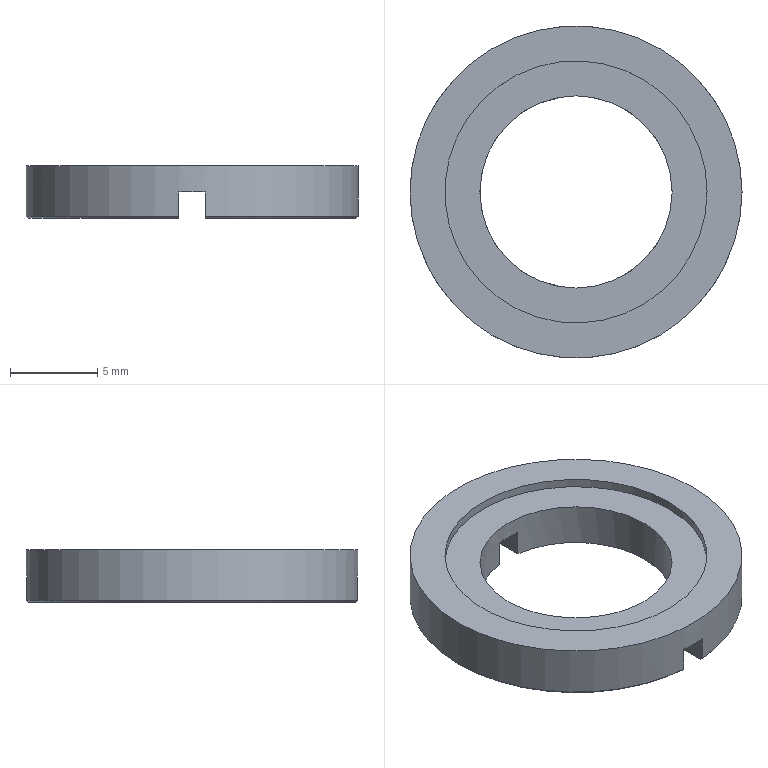Part | NX | 1 solid | 15 faces | box 19 x 19 x 3 mm | volume 506.207 mm3 | plane 10 | cylinder 3 | cone 2 | commonest cylinder face diameters 11 x1 15 x1 19 x1
STEP:
#1=CARTESIAN_POINT('',(-0.75,9.47,1.5));
#2=VERTEX_POINT('',#1);
#3=CARTESIAN_POINT('',(0.75,9.47,1.5));
#4=VERTEX_POINT('',#3);
#5=CARTESIAN_POINT('',(0.,0.,1.5));
#6=DIRECTION('',(0.,0.,-1.));
#7=DIRECTION('',(-1.,0.,0.));
#8=AXIS2_PLACEMENT_3D('',#5,#6,#7);
#9=CIRCLE('',#8,9.5);
#10=EDGE_CURVE('',#2,#4,#9,.T.);
#11=ORIENTED_EDGE('',*,*,#10,.F.);
#12=CARTESIAN_POINT('',(-0.75,9.47,0.12));
#13=VERTEX_POINT('',#12);
#14=CARTESIAN_POINT('',(-0.75,9.47,1.5));
#15=DIRECTION('',(0.,0.,1.));
#16=VECTOR('',#15,1000.);
#17=LINE('',#14,#16);
#18=EDGE_CURVE('',#2,#13,#17,.F.);
#19=ORIENTED_EDGE('',*,*,#18,.T.);
#20=CARTESIAN_POINT('',(-0.75,-9.47,0.12));
#21=VERTEX_POINT('',#20);
#22=CARTESIAN_POINT('',(0.,0.,0.12));
#23=DIRECTION('',(0.,0.,-1.));
#24=DIRECTION('',(-1.,0.,0.));
#25=AXIS2_PLACEMENT_3D('',#22,#23,#24);
#26=CIRCLE('',#25,9.5);
#27=EDGE_CURVE('',#13,#21,#26,.F.);
#28=ORIENTED_EDGE('',*,*,#27,.T.);
#29=CARTESIAN_POINT('',(-0.75,-9.47,1.5));
#30=VERTEX_POINT('',#29);
#31=CARTESIAN_POINT('',(-0.75,-9.47,1.5));
#32=DIRECTION('',(0.,0.,1.));
#33=VECTOR('',#32,1000.);
#34=LINE('',#31,#33);
#35=EDGE_CURVE('',#21,#30,#34,.T.);
#36=ORIENTED_EDGE('',*,*,#35,.T.);
#37=CARTESIAN_POINT('',(0.75,-9.47,1.5));
#38=VERTEX_POINT('',#37);
#39=CARTESIAN_POINT('',(0.,0.,1.5));
#40=DIRECTION('',(0.,0.,-1.));
#41=DIRECTION('',(-1.,0.,0.));
#42=AXIS2_PLACEMENT_3D('',#39,#40,#41);
#43=CIRCLE('',#42,9.5);
#44=EDGE_CURVE('',#38,#30,#43,.T.);
#45=ORIENTED_EDGE('',*,*,#44,.F.);
#46=CARTESIAN_POINT('',(0.75,-9.47,0.12));
#47=VERTEX_POINT('',#46);
#48=CARTESIAN_POINT('',(0.75,-9.47,1.5));
#49=DIRECTION('',(0.,0.,-1.));
#50=VECTOR('',#49,1000.);
#51=LINE('',#48,#50);
#52=EDGE_CURVE('',#38,#47,#51,.T.);
#53=ORIENTED_EDGE('',*,*,#52,.T.);
#54=CARTESIAN_POINT('',(0.75,9.47,0.12));
#55=VERTEX_POINT('',#54);
#56=CARTESIAN_POINT('',(0.,0.,0.12));
#57=DIRECTION('',(0.,0.,-1.));
#58=DIRECTION('',(-1.,0.,0.));
#59=AXIS2_PLACEMENT_3D('',#56,#57,#58);
#60=CIRCLE('',#59,9.5);
#61=EDGE_CURVE('',#47,#55,#60,.F.);
#62=ORIENTED_EDGE('',*,*,#61,.T.);
#63=CARTESIAN_POINT('',(0.75,9.47,1.5));
#64=DIRECTION('',(0.,0.,-1.));
#65=VECTOR('',#64,1000.);
#66=LINE('',#63,#65);
#67=EDGE_CURVE('',#55,#4,#66,.F.);
#68=ORIENTED_EDGE('',*,*,#67,.T.);
#69=EDGE_LOOP('',(#11,#19,#28,#36,#45,#53,#62,#68));
#70=FACE_BOUND('',#69,.T.);
#71=CARTESIAN_POINT('',(-9.5,0.,3.));
#72=VERTEX_POINT('',#71);
#73=CARTESIAN_POINT('',(0.,0.,3.));
#74=DIRECTION('',(0.,0.,-1.));
#75=DIRECTION('',(-1.,0.,0.));
#76=AXIS2_PLACEMENT_3D('',#73,#74,#75);
#77=CIRCLE('',#76,9.5);
#78=EDGE_CURVE('',#72,#72,#77,.T.);
#79=ORIENTED_EDGE('',*,*,#78,.T.);
#80=EDGE_LOOP('',(#79));
#81=FACE_BOUND('',#80,.T.);
#82=CARTESIAN_POINT('',(0.,0.,3.));
#83=DIRECTION('',(0.,0.,-1.));
#84=DIRECTION('',(-1.,0.,0.));
#85=AXIS2_PLACEMENT_3D('',#82,#83,#84);
#86=CYLINDRICAL_SURFACE('',#85,9.5);
#87=ADVANCED_FACE('',(#70,#81),#86,.T.);
#88=ORIENTED_EDGE('',*,*,#61,.F.);
#89=CARTESIAN_POINT('',(0.75,-9.35,0.));
#90=VERTEX_POINT('',#89);
#91=CARTESIAN_POINT('',(0.75,-9.47,0.12));
#92=CARTESIAN_POINT('',(0.75,-9.43,0.08));
#93=CARTESIAN_POINT('',(0.75,-9.39,0.04));
#94=CARTESIAN_POINT('',(0.75,-9.35,0.));
#95=B_SPLINE_CURVE_WITH_KNOTS('',3,(#91,#92,#93,#94),.UNSPECIFIED.,.F.,.F.,(4,4),(0.,0.00017),.UNSPECIFIED.);
#96=EDGE_CURVE('',#47,#90,#95,.T.);
#97=ORIENTED_EDGE('',*,*,#96,.T.);
#98=CARTESIAN_POINT('',(0.75,9.35,0.));
#99=VERTEX_POINT('',#98);
#100=CARTESIAN_POINT('',(0.,0.,0.));
#101=DIRECTION('',(0.,0.,1.));
#102=DIRECTION('',(0.,-1.,0.));
#103=AXIS2_PLACEMENT_3D('',#100,#101,#102);
#104=CIRCLE('',#103,9.38);
#105=EDGE_CURVE('',#90,#99,#104,.T.);
#106=ORIENTED_EDGE('',*,*,#105,.T.);
#107=CARTESIAN_POINT('',(0.75,9.35,0.));
#108=CARTESIAN_POINT('',(0.75,9.39,0.04));
#109=CARTESIAN_POINT('',(0.75,9.43,0.08));
#110=CARTESIAN_POINT('',(0.75,9.47,0.12));
#111=B_SPLINE_CURVE_WITH_KNOTS('',3,(#107,#108,#109,#110),.UNSPECIFIED.,.F.,.F.,(4,4),(0.,0.00017),.UNSPECIFIED.);
#112=EDGE_CURVE('',#99,#55,#111,.T.);
#113=ORIENTED_EDGE('',*,*,#112,.T.);
#114=EDGE_LOOP('',(#88,#97,#106,#113));
#115=FACE_BOUND('',#114,.T.);
#116=CARTESIAN_POINT('',(0.,0.,0.12));
#117=DIRECTION('',(0.,0.,1.));
#118=DIRECTION('',(0.,-1.,0.));
#119=AXIS2_PLACEMENT_3D('',#116,#117,#118);
#120=CONICAL_SURFACE('',#119,9.5,0.7854);
#121=ADVANCED_FACE('',(#115),#120,.T.);
#122=CARTESIAN_POINT('',(-0.75,9.35,0.));
#123=VERTEX_POINT('',#122);
#124=CARTESIAN_POINT('',(-0.75,9.47,0.12));
#125=CARTESIAN_POINT('',(-0.75,9.43,0.08));
#126=CARTESIAN_POINT('',(-0.75,9.39,0.04));
#127=CARTESIAN_POINT('',(-0.75,9.35,0.));
#128=B_SPLINE_CURVE_WITH_KNOTS('',3,(#124,#125,#126,#127),.UNSPECIFIED.,.F.,.F.,(4,4),(0.,0.00017),.UNSPECIFIED.);
#129=EDGE_CURVE('',#13,#123,#128,.T.);
#130=ORIENTED_EDGE('',*,*,#129,.T.);
#131=CARTESIAN_POINT('',(-0.75,-9.35,0.));
#132=VERTEX_POINT('',#131);
#133=CARTESIAN_POINT('',(0.,0.,0.));
#134=DIRECTION('',(0.,0.,1.));
#135=DIRECTION('',(0.,-1.,0.));
#136=AXIS2_PLACEMENT_3D('',#133,#134,#135);
#137=CIRCLE('',#136,9.38);
#138=EDGE_CURVE('',#123,#132,#137,.T.);
#139=ORIENTED_EDGE('',*,*,#138,.T.);
#140=CARTESIAN_POINT('',(-0.75,-9.35,0.));
#141=CARTESIAN_POINT('',(-0.75,-9.39,0.04));
#142=CARTESIAN_POINT('',(-0.75,-9.43,0.08));
#143=CARTESIAN_POINT('',(-0.75,-9.47,0.12));
#144=B_SPLINE_CURVE_WITH_KNOTS('',3,(#140,#141,#142,#143),.UNSPECIFIED.,.F.,.F.,(4,4),(0.,0.00017),.UNSPECIFIED.);
#145=EDGE_CURVE('',#132,#21,#144,.T.);
#146=ORIENTED_EDGE('',*,*,#145,.T.);
#147=ORIENTED_EDGE('',*,*,#27,.F.);
#148=EDGE_LOOP('',(#130,#139,#146,#147));
#149=FACE_BOUND('',#148,.T.);
#150=CARTESIAN_POINT('',(0.,0.,0.12));
#151=DIRECTION('',(0.,0.,1.));
#152=DIRECTION('',(0.,-1.,0.));
#153=AXIS2_PLACEMENT_3D('',#150,#151,#152);
#154=CONICAL_SURFACE('',#153,9.5,0.7854);
#155=ADVANCED_FACE('',(#149),#154,.T.);
#156=CARTESIAN_POINT('',(7.5,0.,3.));
#157=VERTEX_POINT('',#156);
#158=CARTESIAN_POINT('',(0.,0.,3.));
#159=DIRECTION('',(0.,0.,1.));
#160=DIRECTION('',(1.,0.,0.));
#161=AXIS2_PLACEMENT_3D('',#158,#159,#160);
#162=CIRCLE('',#161,7.5);
#163=EDGE_CURVE('',#157,#157,#162,.F.);
#164=ORIENTED_EDGE('',*,*,#163,.T.);
#165=EDGE_LOOP('',(#164));
#166=FACE_BOUND('',#165,.T.);
#167=ORIENTED_EDGE('',*,*,#78,.F.);
#168=EDGE_LOOP('',(#167));
#169=FACE_BOUND('',#168,.T.);
#170=CARTESIAN_POINT('',(0.,0.,3.));
#171=DIRECTION('',(0.,0.,1.));
#172=DIRECTION('',(1.,0.,0.));
#173=AXIS2_PLACEMENT_3D('',#170,#171,#172);
#174=PLANE('',#173);
#175=ADVANCED_FACE('',(#166,#169),#174,.T.);
#176=CARTESIAN_POINT('',(0.75,-5.449,0.));
#177=VERTEX_POINT('',#176);
#178=CARTESIAN_POINT('',(0.75,0.,0.));
#179=DIRECTION('',(0.,1.,0.));
#180=VECTOR('',#179,1000.);
#181=LINE('',#178,#180);
#182=EDGE_CURVE('',#177,#90,#181,.F.);
#183=ORIENTED_EDGE('',*,*,#182,.F.);
#184=CARTESIAN_POINT('',(0.75,5.449,0.));
#185=VERTEX_POINT('',#184);
#186=CARTESIAN_POINT('',(0.,0.,0.));
#187=DIRECTION('',(0.,0.,1.));
#188=DIRECTION('',(1.,0.,0.));
#189=AXIS2_PLACEMENT_3D('',#186,#187,#188);
#190=CIRCLE('',#189,5.5);
#191=EDGE_CURVE('',#185,#177,#190,.F.);
#192=ORIENTED_EDGE('',*,*,#191,.F.);
#193=CARTESIAN_POINT('',(0.75,0.,0.));
#194=DIRECTION('',(0.,1.,0.));
#195=VECTOR('',#194,1000.);
#196=LINE('',#193,#195);
#197=EDGE_CURVE('',#99,#185,#196,.F.);
#198=ORIENTED_EDGE('',*,*,#197,.F.);
#199=ORIENTED_EDGE('',*,*,#105,.F.);
#200=EDGE_LOOP('',(#183,#192,#198,#199));
#201=FACE_BOUND('',#200,.T.);
#202=CARTESIAN_POINT('',(0.,0.,0.));
#203=DIRECTION('',(0.,0.,1.));
#204=DIRECTION('',(1.,0.,0.));
#205=AXIS2_PLACEMENT_3D('',#202,#203,#204);
#206=PLANE('',#205);
#207=ADVANCED_FACE('',(#201),#206,.F.);
#208=CARTESIAN_POINT('',(-0.75,5.449,0.));
#209=VERTEX_POINT('',#208);
#210=CARTESIAN_POINT('',(-0.75,0.,0.));
#211=DIRECTION('',(0.,1.,0.));
#212=VECTOR('',#211,1000.);
#213=LINE('',#210,#212);
#214=EDGE_CURVE('',#209,#123,#213,.T.);
#215=ORIENTED_EDGE('',*,*,#214,.F.);
#216=CARTESIAN_POINT('',(-0.75,-5.449,0.));
#217=VERTEX_POINT('',#216);
#218=CARTESIAN_POINT('',(0.,0.,0.));
#219=DIRECTION('',(0.,0.,1.));
#220=DIRECTION('',(1.,0.,0.));
#221=AXIS2_PLACEMENT_3D('',#218,#219,#220);
#222=CIRCLE('',#221,5.5);
#223=EDGE_CURVE('',#217,#209,#222,.F.);
#224=ORIENTED_EDGE('',*,*,#223,.F.);
#225=CARTESIAN_POINT('',(-0.75,0.,0.));
#226=DIRECTION('',(0.,1.,0.));
#227=VECTOR('',#226,1000.);
#228=LINE('',#225,#227);
#229=EDGE_CURVE('',#132,#217,#228,.T.);
#230=ORIENTED_EDGE('',*,*,#229,.F.);
#231=ORIENTED_EDGE('',*,*,#138,.F.);
#232=EDGE_LOOP('',(#215,#224,#230,#231));
#233=FACE_BOUND('',#232,.T.);
#234=CARTESIAN_POINT('',(0.,0.,0.));
#235=DIRECTION('',(0.,0.,1.));
#236=DIRECTION('',(1.,0.,0.));
#237=AXIS2_PLACEMENT_3D('',#234,#235,#236);
#238=PLANE('',#237);
#239=ADVANCED_FACE('',(#233),#238,.F.);
#240=ORIENTED_EDGE('',*,*,#163,.F.);
#241=EDGE_LOOP('',(#240));
#242=FACE_BOUND('',#241,.T.);
#243=CARTESIAN_POINT('',(7.5,0.,2.5));
#244=VERTEX_POINT('',#243);
#245=CARTESIAN_POINT('',(0.,0.,2.5));
#246=DIRECTION('',(0.,0.,1.));
#247=DIRECTION('',(1.,0.,0.));
#248=AXIS2_PLACEMENT_3D('',#245,#246,#247);
#249=CIRCLE('',#248,7.5);
#250=EDGE_CURVE('',#244,#244,#249,.T.);
#251=ORIENTED_EDGE('',*,*,#250,.F.);
#252=EDGE_LOOP('',(#251));
#253=FACE_BOUND('',#252,.T.);
#254=CARTESIAN_POINT('',(0.,0.,2.5));
#255=DIRECTION('',(0.,0.,1.));
#256=DIRECTION('',(1.,0.,0.));
#257=AXIS2_PLACEMENT_3D('',#254,#255,#256);
#258=CYLINDRICAL_SURFACE('',#257,7.5);
#259=ADVANCED_FACE('',(#242,#253),#258,.F.);
#260=ORIENTED_EDGE('',*,*,#96,.F.);
#261=ORIENTED_EDGE('',*,*,#52,.F.);
#262=CARTESIAN_POINT('',(0.75,-5.449,1.5));
#263=VERTEX_POINT('',#262);
#264=CARTESIAN_POINT('',(0.75,10.835,1.5));
#265=DIRECTION('',(0.,1.,0.));
#266=VECTOR('',#265,1000.);
#267=LINE('',#264,#266);
#268=EDGE_CURVE('',#263,#38,#267,.F.);
#269=ORIENTED_EDGE('',*,*,#268,.F.);
#270=CARTESIAN_POINT('',(0.75,-5.449,1.5));
#271=DIRECTION('',(0.,0.,-1.));
#272=VECTOR('',#271,1000.);
#273=LINE('',#270,#272);
#274=EDGE_CURVE('',#177,#263,#273,.F.);
#275=ORIENTED_EDGE('',*,*,#274,.F.);
#276=ORIENTED_EDGE('',*,*,#182,.T.);
#277=EDGE_LOOP('',(#260,#261,#269,#275,#276));
#278=FACE_BOUND('',#277,.T.);
#279=CARTESIAN_POINT('',(0.75,10.835,1.5));
#280=DIRECTION('',(1.,0.,0.));
#281=DIRECTION('',(0.,0.,-1.));
#282=AXIS2_PLACEMENT_3D('',#279,#280,#281);
#283=PLANE('',#282);
#284=ADVANCED_FACE('',(#278),#283,.F.);
#285=CARTESIAN_POINT('',(5.5,0.,2.5));
#286=VERTEX_POINT('',#285);
#287=CARTESIAN_POINT('',(0.,0.,2.5));
#288=DIRECTION('',(0.,0.,1.));
#289=DIRECTION('',(1.,0.,0.));
#290=AXIS2_PLACEMENT_3D('',#287,#288,#289);
#291=CIRCLE('',#290,5.5);
#292=EDGE_CURVE('',#286,#286,#291,.F.);
#293=ORIENTED_EDGE('',*,*,#292,.F.);
#294=EDGE_LOOP('',(#293));
#295=FACE_BOUND('',#294,.T.);
#296=ORIENTED_EDGE('',*,*,#274,.T.);
#297=CARTESIAN_POINT('',(-0.75,-5.449,1.5));
#298=VERTEX_POINT('',#297);
#299=CARTESIAN_POINT('',(0.,0.,1.5));
#300=DIRECTION('',(0.,0.,1.));
#301=DIRECTION('',(1.,0.,0.));
#302=AXIS2_PLACEMENT_3D('',#299,#300,#301);
#303=CIRCLE('',#302,5.5);
#304=EDGE_CURVE('',#298,#263,#303,.T.);
#305=ORIENTED_EDGE('',*,*,#304,.F.);
#306=CARTESIAN_POINT('',(-0.75,-5.449,0.));
#307=DIRECTION('',(0.,0.,1.));
#308=VECTOR('',#307,1000.);
#309=LINE('',#306,#308);
#310=EDGE_CURVE('',#217,#298,#309,.T.);
#311=ORIENTED_EDGE('',*,*,#310,.F.);
#312=ORIENTED_EDGE('',*,*,#223,.T.);
#313=CARTESIAN_POINT('',(-0.75,5.449,1.5));
#314=VERTEX_POINT('',#313);
#315=CARTESIAN_POINT('',(-0.75,5.449,0.));
#316=DIRECTION('',(0.,0.,1.));
#317=VECTOR('',#316,1000.);
#318=LINE('',#315,#317);
#319=EDGE_CURVE('',#314,#209,#318,.F.);
#320=ORIENTED_EDGE('',*,*,#319,.F.);
#321=CARTESIAN_POINT('',(0.75,5.449,1.5));
#322=VERTEX_POINT('',#321);
#323=CARTESIAN_POINT('',(0.,0.,1.5));
#324=DIRECTION('',(0.,0.,1.));
#325=DIRECTION('',(1.,0.,0.));
#326=AXIS2_PLACEMENT_3D('',#323,#324,#325);
#327=CIRCLE('',#326,5.5);
#328=EDGE_CURVE('',#322,#314,#327,.T.);
#329=ORIENTED_EDGE('',*,*,#328,.F.);
#330=CARTESIAN_POINT('',(0.75,5.449,0.));
#331=DIRECTION('',(0.,0.,1.));
#332=VECTOR('',#331,1000.);
#333=LINE('',#330,#332);
#334=EDGE_CURVE('',#185,#322,#333,.T.);
#335=ORIENTED_EDGE('',*,*,#334,.F.);
#336=ORIENTED_EDGE('',*,*,#191,.T.);
#337=EDGE_LOOP('',(#296,#305,#311,#312,#320,#329,#335,#336));
#338=FACE_BOUND('',#337,.T.);
#339=CARTESIAN_POINT('',(0.,0.,0.));
#340=DIRECTION('',(0.,0.,1.));
#341=DIRECTION('',(1.,0.,0.));
#342=AXIS2_PLACEMENT_3D('',#339,#340,#341);
#343=CYLINDRICAL_SURFACE('',#342,5.5);
#344=ADVANCED_FACE('',(#295,#338),#343,.F.);
#345=ORIENTED_EDGE('',*,*,#67,.F.);
#346=ORIENTED_EDGE('',*,*,#112,.F.);
#347=ORIENTED_EDGE('',*,*,#197,.T.);
#348=ORIENTED_EDGE('',*,*,#334,.T.);
#349=CARTESIAN_POINT('',(0.75,10.835,1.5));
#350=DIRECTION('',(0.,1.,0.));
#351=VECTOR('',#350,1000.);
#352=LINE('',#349,#351);
#353=EDGE_CURVE('',#4,#322,#352,.F.);
#354=ORIENTED_EDGE('',*,*,#353,.F.);
#355=EDGE_LOOP('',(#345,#346,#347,#348,#354));
#356=FACE_BOUND('',#355,.T.);
#357=CARTESIAN_POINT('',(0.75,10.835,1.5));
#358=DIRECTION('',(1.,0.,0.));
#359=DIRECTION('',(0.,0.,-1.));
#360=AXIS2_PLACEMENT_3D('',#357,#358,#359);
#361=PLANE('',#360);
#362=ADVANCED_FACE('',(#356),#361,.F.);
#363=ORIENTED_EDGE('',*,*,#129,.F.);
#364=ORIENTED_EDGE('',*,*,#18,.F.);
#365=CARTESIAN_POINT('',(-0.75,10.835,1.5));
#366=DIRECTION('',(0.,1.,0.));
#367=VECTOR('',#366,1000.);
#368=LINE('',#365,#367);
#369=EDGE_CURVE('',#314,#2,#368,.T.);
#370=ORIENTED_EDGE('',*,*,#369,.F.);
#371=ORIENTED_EDGE('',*,*,#319,.T.);
#372=ORIENTED_EDGE('',*,*,#214,.T.);
#373=EDGE_LOOP('',(#363,#364,#370,#371,#372));
#374=FACE_BOUND('',#373,.T.);
#375=CARTESIAN_POINT('',(-0.75,10.835,1.5));
#376=DIRECTION('',(-1.,0.,0.));
#377=DIRECTION('',(0.,0.,1.));
#378=AXIS2_PLACEMENT_3D('',#375,#376,#377);
#379=PLANE('',#378);
#380=ADVANCED_FACE('',(#374),#379,.F.);
#381=ORIENTED_EDGE('',*,*,#35,.F.);
#382=ORIENTED_EDGE('',*,*,#145,.F.);
#383=ORIENTED_EDGE('',*,*,#229,.T.);
#384=ORIENTED_EDGE('',*,*,#310,.T.);
#385=CARTESIAN_POINT('',(-0.75,10.835,1.5));
#386=DIRECTION('',(0.,1.,0.));
#387=VECTOR('',#386,1000.);
#388=LINE('',#385,#387);
#389=EDGE_CURVE('',#30,#298,#388,.T.);
#390=ORIENTED_EDGE('',*,*,#389,.F.);
#391=EDGE_LOOP('',(#381,#382,#383,#384,#390));
#392=FACE_BOUND('',#391,.T.);
#393=CARTESIAN_POINT('',(-0.75,10.835,1.5));
#394=DIRECTION('',(-1.,0.,0.));
#395=DIRECTION('',(0.,0.,1.));
#396=AXIS2_PLACEMENT_3D('',#393,#394,#395);
#397=PLANE('',#396);
#398=ADVANCED_FACE('',(#392),#397,.F.);
#399=ORIENTED_EDGE('',*,*,#292,.T.);
#400=EDGE_LOOP('',(#399));
#401=FACE_BOUND('',#400,.T.);
#402=ORIENTED_EDGE('',*,*,#250,.T.);
#403=EDGE_LOOP('',(#402));
#404=FACE_BOUND('',#403,.T.);
#405=CARTESIAN_POINT('',(0.,0.,2.5));
#406=DIRECTION('',(0.,0.,1.));
#407=DIRECTION('',(1.,0.,0.));
#408=AXIS2_PLACEMENT_3D('',#405,#406,#407);
#409=PLANE('',#408);
#410=ADVANCED_FACE('',(#401,#404),#409,.T.);
#411=ORIENTED_EDGE('',*,*,#304,.T.);
#412=ORIENTED_EDGE('',*,*,#268,.T.);
#413=ORIENTED_EDGE('',*,*,#44,.T.);
#414=ORIENTED_EDGE('',*,*,#389,.T.);
#415=EDGE_LOOP('',(#411,#412,#413,#414));
#416=FACE_BOUND('',#415,.T.);
#417=CARTESIAN_POINT('',(0.75,-11.779,1.5));
#418=DIRECTION('',(0.,0.,-1.));
#419=DIRECTION('',(-1.,0.,0.));
#420=AXIS2_PLACEMENT_3D('',#417,#418,#419);
#421=PLANE('',#420);
#422=ADVANCED_FACE('',(#416),#421,.T.);
#423=ORIENTED_EDGE('',*,*,#328,.T.);
#424=ORIENTED_EDGE('',*,*,#369,.T.);
#425=ORIENTED_EDGE('',*,*,#10,.T.);
#426=ORIENTED_EDGE('',*,*,#353,.T.);
#427=EDGE_LOOP('',(#423,#424,#425,#426));
#428=FACE_BOUND('',#427,.T.);
#429=CARTESIAN_POINT('',(0.75,-11.779,1.5));
#430=DIRECTION('',(0.,0.,-1.));
#431=DIRECTION('',(-1.,0.,0.));
#432=AXIS2_PLACEMENT_3D('',#429,#430,#431);
#433=PLANE('',#432);
#434=ADVANCED_FACE('',(#428),#433,.T.);
#435=CLOSED_SHELL('',(#87,#121,#155,#175,#207,#239,#259,#284,#344,#362,#380,#398,#410,#422,#434));
#436=MANIFOLD_SOLID_BREP('',#435);
#437=(LENGTH_UNIT()NAMED_UNIT(*)SI_UNIT(.MILLI.,.METRE.));
#438=UNCERTAINTY_MEASURE_WITH_UNIT(LENGTH_MEASURE(0.0508),#437,'','');
#439=(NAMED_UNIT(*)PLANE_ANGLE_UNIT()SI_UNIT($,.RADIAN.));
#440=(NAMED_UNIT(*)SI_UNIT($,.STERADIAN.)SOLID_ANGLE_UNIT());
#441=(GEOMETRIC_REPRESENTATION_CONTEXT(3)GLOBAL_UNCERTAINTY_ASSIGNED_CONTEXT((#438))GLOBAL_UNIT_ASSIGNED_CONTEXT((#437,#439,#440))REPRESENTATION_CONTEXT('',''));
#442=ADVANCED_BREP_SHAPE_REPRESENTATION('',(#436),#441);